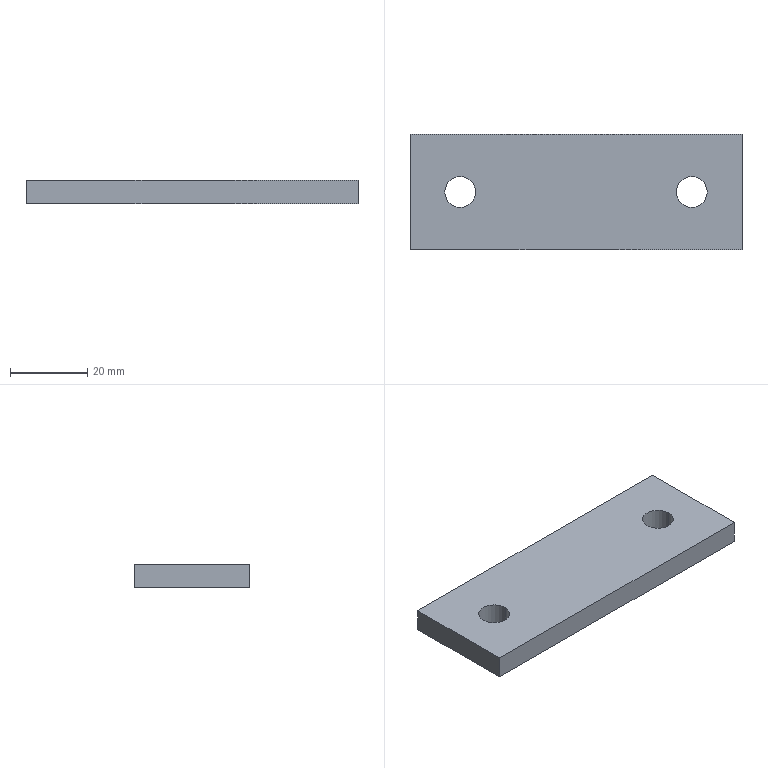Part | SolidWorks | features Extrusion 1, ICE 1 | 1 solid | 10 faces | box 86 x 30 x 6 mm | volume 14877 mm3 | plane 6 | cylinder 4 | commonest cylinder face diameters 8 x4
STEP:
#1=CARTESIAN_POINT('',(-26.,0.,0.));
#2=VERTEX_POINT('',#1);
#3=CARTESIAN_POINT('',(-34.,0.,0.));
#4=VERTEX_POINT('',#3);
#5=CARTESIAN_POINT('',(-30.,0.,0.));
#6=DIRECTION('',(0.,0.,-1.));
#7=DIRECTION('',(-1.,0.,0.));
#8=AXIS2_PLACEMENT_3D('',#5,#6,#7);
#9=CIRCLE('',#8,4.);
#10=EDGE_CURVE('',#2,#4,#9,.T.);
#11=ORIENTED_EDGE('',*,*,#10,.T.);
#12=CARTESIAN_POINT('',(-34.,0.,6.));
#13=VERTEX_POINT('',#12);
#14=CARTESIAN_POINT('',(-34.,0.,-4.));
#15=DIRECTION('',(0.,0.,1.));
#16=VECTOR('',#15,1000.);
#17=LINE('',#14,#16);
#18=EDGE_CURVE('',#4,#13,#17,.T.);
#19=ORIENTED_EDGE('',*,*,#18,.T.);
#20=CARTESIAN_POINT('',(-26.,0.,6.));
#21=VERTEX_POINT('',#20);
#22=CARTESIAN_POINT('',(-30.,0.,6.));
#23=DIRECTION('',(0.,0.,1.));
#24=DIRECTION('',(1.,0.,0.));
#25=AXIS2_PLACEMENT_3D('',#22,#23,#24);
#26=CIRCLE('',#25,4.);
#27=EDGE_CURVE('',#13,#21,#26,.T.);
#28=ORIENTED_EDGE('',*,*,#27,.T.);
#29=CARTESIAN_POINT('',(-26.,0.,-4.));
#30=DIRECTION('',(0.,0.,1.));
#31=VECTOR('',#30,1000.);
#32=LINE('',#29,#31);
#33=EDGE_CURVE('',#2,#21,#32,.T.);
#34=ORIENTED_EDGE('',*,*,#33,.F.);
#35=EDGE_LOOP('',(#11,#19,#28,#34));
#36=FACE_OUTER_BOUND('',#35,.T.);
#37=CARTESIAN_POINT('',(-30.,0.,-4.));
#38=DIRECTION('',(0.,0.,1.));
#39=DIRECTION('',(1.,0.,0.));
#40=AXIS2_PLACEMENT_3D('',#37,#38,#39);
#41=CYLINDRICAL_SURFACE('',#40,4.);
#42=ADVANCED_FACE('',(#36),#41,.F.);
#43=CARTESIAN_POINT('',(34.,0.,0.));
#44=VERTEX_POINT('',#43);
#45=CARTESIAN_POINT('',(26.,0.,0.));
#46=VERTEX_POINT('',#45);
#47=CARTESIAN_POINT('',(30.,0.,0.));
#48=DIRECTION('',(0.,0.,-1.));
#49=DIRECTION('',(-1.,0.,0.));
#50=AXIS2_PLACEMENT_3D('',#47,#48,#49);
#51=CIRCLE('',#50,4.);
#52=EDGE_CURVE('',#44,#46,#51,.T.);
#53=ORIENTED_EDGE('',*,*,#52,.T.);
#54=CARTESIAN_POINT('',(26.,0.,6.));
#55=VERTEX_POINT('',#54);
#56=CARTESIAN_POINT('',(26.,0.,-4.));
#57=DIRECTION('',(0.,0.,1.));
#58=VECTOR('',#57,1000.);
#59=LINE('',#56,#58);
#60=EDGE_CURVE('',#46,#55,#59,.T.);
#61=ORIENTED_EDGE('',*,*,#60,.T.);
#62=CARTESIAN_POINT('',(34.,0.,6.));
#63=VERTEX_POINT('',#62);
#64=CARTESIAN_POINT('',(30.,0.,6.));
#65=DIRECTION('',(0.,0.,1.));
#66=DIRECTION('',(1.,0.,0.));
#67=AXIS2_PLACEMENT_3D('',#64,#65,#66);
#68=CIRCLE('',#67,4.);
#69=EDGE_CURVE('',#55,#63,#68,.T.);
#70=ORIENTED_EDGE('',*,*,#69,.T.);
#71=CARTESIAN_POINT('',(34.,0.,-4.));
#72=DIRECTION('',(0.,0.,1.));
#73=VECTOR('',#72,1000.);
#74=LINE('',#71,#73);
#75=EDGE_CURVE('',#44,#63,#74,.T.);
#76=ORIENTED_EDGE('',*,*,#75,.F.);
#77=EDGE_LOOP('',(#53,#61,#70,#76));
#78=FACE_OUTER_BOUND('',#77,.T.);
#79=CARTESIAN_POINT('',(30.,0.,-4.));
#80=DIRECTION('',(0.,0.,1.));
#81=DIRECTION('',(1.,0.,0.));
#82=AXIS2_PLACEMENT_3D('',#79,#80,#81);
#83=CYLINDRICAL_SURFACE('',#82,4.);
#84=ADVANCED_FACE('',(#78),#83,.F.);
#85=CARTESIAN_POINT('',(-43.,15.,0.));
#86=VERTEX_POINT('',#85);
#87=CARTESIAN_POINT('',(-43.,-15.,0.));
#88=VERTEX_POINT('',#87);
#89=CARTESIAN_POINT('',(-43.,15.,0.));
#90=DIRECTION('',(0.,-1.,0.));
#91=VECTOR('',#90,1000.);
#92=LINE('',#89,#91);
#93=EDGE_CURVE('',#86,#88,#92,.T.);
#94=ORIENTED_EDGE('',*,*,#93,.T.);
#95=CARTESIAN_POINT('',(-43.,-15.,6.));
#96=VERTEX_POINT('',#95);
#97=CARTESIAN_POINT('',(-43.,-15.,6.));
#98=DIRECTION('',(0.,0.,-1.));
#99=VECTOR('',#98,1000.);
#100=LINE('',#97,#99);
#101=EDGE_CURVE('',#96,#88,#100,.T.);
#102=ORIENTED_EDGE('',*,*,#101,.F.);
#103=CARTESIAN_POINT('',(-43.,15.,6.));
#104=VERTEX_POINT('',#103);
#105=CARTESIAN_POINT('',(-43.,15.,6.));
#106=DIRECTION('',(0.,-1.,0.));
#107=VECTOR('',#106,1000.);
#108=LINE('',#105,#107);
#109=EDGE_CURVE('',#104,#96,#108,.T.);
#110=ORIENTED_EDGE('',*,*,#109,.F.);
#111=CARTESIAN_POINT('',(-43.,15.,6.));
#112=DIRECTION('',(0.,0.,-1.));
#113=VECTOR('',#112,1000.);
#114=LINE('',#111,#113);
#115=EDGE_CURVE('',#104,#86,#114,.T.);
#116=ORIENTED_EDGE('',*,*,#115,.T.);
#117=EDGE_LOOP('',(#94,#102,#110,#116));
#118=FACE_OUTER_BOUND('',#117,.T.);
#119=CARTESIAN_POINT('',(-43.,15.,6.));
#120=DIRECTION('',(1.,0.,0.));
#121=DIRECTION('',(0.,1.,0.));
#122=AXIS2_PLACEMENT_3D('',#119,#120,#121);
#123=PLANE('',#122);
#124=ADVANCED_FACE('',(#118),#123,.F.);
#125=CARTESIAN_POINT('',(43.,-15.,0.));
#126=VERTEX_POINT('',#125);
#127=CARTESIAN_POINT('',(43.,-15.,0.));
#128=DIRECTION('',(1.,0.,0.));
#129=VECTOR('',#128,1000.);
#130=LINE('',#127,#129);
#131=EDGE_CURVE('',#88,#126,#130,.T.);
#132=ORIENTED_EDGE('',*,*,#131,.T.);
#133=CARTESIAN_POINT('',(43.,-15.,6.));
#134=VERTEX_POINT('',#133);
#135=CARTESIAN_POINT('',(43.,-15.,6.));
#136=DIRECTION('',(0.,0.,-1.));
#137=VECTOR('',#136,1000.);
#138=LINE('',#135,#137);
#139=EDGE_CURVE('',#134,#126,#138,.T.);
#140=ORIENTED_EDGE('',*,*,#139,.F.);
#141=CARTESIAN_POINT('',(43.,-15.,6.));
#142=DIRECTION('',(1.,0.,0.));
#143=VECTOR('',#142,1000.);
#144=LINE('',#141,#143);
#145=EDGE_CURVE('',#96,#134,#144,.T.);
#146=ORIENTED_EDGE('',*,*,#145,.F.);
#147=ORIENTED_EDGE('',*,*,#101,.T.);
#148=EDGE_LOOP('',(#132,#140,#146,#147));
#149=FACE_OUTER_BOUND('',#148,.T.);
#150=CARTESIAN_POINT('',(43.,-15.,6.));
#151=DIRECTION('',(0.,1.,0.));
#152=DIRECTION('',(-1.,0.,0.));
#153=AXIS2_PLACEMENT_3D('',#150,#151,#152);
#154=PLANE('',#153);
#155=ADVANCED_FACE('',(#149),#154,.F.);
#156=CARTESIAN_POINT('',(43.,15.,0.));
#157=VERTEX_POINT('',#156);
#158=CARTESIAN_POINT('',(43.,15.,0.));
#159=DIRECTION('',(0.,1.,0.));
#160=VECTOR('',#159,1000.);
#161=LINE('',#158,#160);
#162=EDGE_CURVE('',#126,#157,#161,.T.);
#163=ORIENTED_EDGE('',*,*,#162,.T.);
#164=CARTESIAN_POINT('',(43.,15.,6.));
#165=VERTEX_POINT('',#164);
#166=CARTESIAN_POINT('',(43.,15.,6.));
#167=DIRECTION('',(0.,0.,-1.));
#168=VECTOR('',#167,1000.);
#169=LINE('',#166,#168);
#170=EDGE_CURVE('',#165,#157,#169,.T.);
#171=ORIENTED_EDGE('',*,*,#170,.F.);
#172=CARTESIAN_POINT('',(43.,15.,6.));
#173=DIRECTION('',(0.,1.,0.));
#174=VECTOR('',#173,1000.);
#175=LINE('',#172,#174);
#176=EDGE_CURVE('',#134,#165,#175,.T.);
#177=ORIENTED_EDGE('',*,*,#176,.F.);
#178=ORIENTED_EDGE('',*,*,#139,.T.);
#179=EDGE_LOOP('',(#163,#171,#177,#178));
#180=FACE_OUTER_BOUND('',#179,.T.);
#181=CARTESIAN_POINT('',(43.,15.,6.));
#182=DIRECTION('',(-1.,0.,0.));
#183=DIRECTION('',(0.,-1.,0.));
#184=AXIS2_PLACEMENT_3D('',#181,#182,#183);
#185=PLANE('',#184);
#186=ADVANCED_FACE('',(#180),#185,.F.);
#187=CARTESIAN_POINT('',(43.,15.,0.));
#188=DIRECTION('',(-1.,0.,0.));
#189=VECTOR('',#188,1000.);
#190=LINE('',#187,#189);
#191=EDGE_CURVE('',#157,#86,#190,.T.);
#192=ORIENTED_EDGE('',*,*,#191,.T.);
#193=ORIENTED_EDGE('',*,*,#115,.F.);
#194=CARTESIAN_POINT('',(43.,15.,6.));
#195=DIRECTION('',(-1.,0.,0.));
#196=VECTOR('',#195,1000.);
#197=LINE('',#194,#196);
#198=EDGE_CURVE('',#165,#104,#197,.T.);
#199=ORIENTED_EDGE('',*,*,#198,.F.);
#200=ORIENTED_EDGE('',*,*,#170,.T.);
#201=EDGE_LOOP('',(#192,#193,#199,#200));
#202=FACE_OUTER_BOUND('',#201,.T.);
#203=CARTESIAN_POINT('',(43.,15.,6.));
#204=DIRECTION('',(0.,-1.,0.));
#205=DIRECTION('',(1.,0.,0.));
#206=AXIS2_PLACEMENT_3D('',#203,#204,#205);
#207=PLANE('',#206);
#208=ADVANCED_FACE('',(#202),#207,.F.);
#209=CARTESIAN_POINT('',(-30.,0.,6.));
#210=DIRECTION('',(0.,0.,1.));
#211=DIRECTION('',(1.,0.,0.));
#212=AXIS2_PLACEMENT_3D('',#209,#210,#211);
#213=CIRCLE('',#212,4.);
#214=EDGE_CURVE('',#21,#13,#213,.T.);
#215=ORIENTED_EDGE('',*,*,#214,.F.);
#216=ORIENTED_EDGE('',*,*,#27,.F.);
#217=EDGE_LOOP('',(#215,#216));
#218=FACE_BOUND('',#217,.T.);
#219=CARTESIAN_POINT('',(30.,0.,6.));
#220=DIRECTION('',(0.,0.,1.));
#221=DIRECTION('',(1.,0.,0.));
#222=AXIS2_PLACEMENT_3D('',#219,#220,#221);
#223=CIRCLE('',#222,4.);
#224=EDGE_CURVE('',#63,#55,#223,.T.);
#225=ORIENTED_EDGE('',*,*,#224,.F.);
#226=ORIENTED_EDGE('',*,*,#69,.F.);
#227=EDGE_LOOP('',(#225,#226));
#228=FACE_BOUND('',#227,.T.);
#229=ORIENTED_EDGE('',*,*,#109,.T.);
#230=ORIENTED_EDGE('',*,*,#145,.T.);
#231=ORIENTED_EDGE('',*,*,#176,.T.);
#232=ORIENTED_EDGE('',*,*,#198,.T.);
#233=EDGE_LOOP('',(#229,#230,#231,#232));
#234=FACE_OUTER_BOUND('',#233,.T.);
#235=CARTESIAN_POINT('',(0.,0.,6.));
#236=DIRECTION('',(0.,0.,-1.));
#237=DIRECTION('',(-1.,0.,0.));
#238=AXIS2_PLACEMENT_3D('',#235,#236,#237);
#239=PLANE('',#238);
#240=ADVANCED_FACE('',(#218,#228,#234),#239,.F.);
#241=ORIENTED_EDGE('',*,*,#10,.F.);
#242=CARTESIAN_POINT('',(-30.,0.,0.));
#243=DIRECTION('',(0.,0.,-1.));
#244=DIRECTION('',(-1.,0.,0.));
#245=AXIS2_PLACEMENT_3D('',#242,#243,#244);
#246=CIRCLE('',#245,4.);
#247=EDGE_CURVE('',#4,#2,#246,.T.);
#248=ORIENTED_EDGE('',*,*,#247,.F.);
#249=EDGE_LOOP('',(#241,#248));
#250=FACE_BOUND('',#249,.T.);
#251=ORIENTED_EDGE('',*,*,#52,.F.);
#252=CARTESIAN_POINT('',(30.,0.,0.));
#253=DIRECTION('',(0.,0.,-1.));
#254=DIRECTION('',(-1.,0.,0.));
#255=AXIS2_PLACEMENT_3D('',#252,#253,#254);
#256=CIRCLE('',#255,4.);
#257=EDGE_CURVE('',#46,#44,#256,.T.);
#258=ORIENTED_EDGE('',*,*,#257,.F.);
#259=EDGE_LOOP('',(#251,#258));
#260=FACE_BOUND('',#259,.T.);
#261=ORIENTED_EDGE('',*,*,#93,.F.);
#262=ORIENTED_EDGE('',*,*,#191,.F.);
#263=ORIENTED_EDGE('',*,*,#162,.F.);
#264=ORIENTED_EDGE('',*,*,#131,.F.);
#265=EDGE_LOOP('',(#261,#262,#263,#264));
#266=FACE_OUTER_BOUND('',#265,.T.);
#267=CARTESIAN_POINT('',(0.,0.,0.));
#268=DIRECTION('',(0.,0.,-1.));
#269=DIRECTION('',(-1.,0.,0.));
#270=AXIS2_PLACEMENT_3D('',#267,#268,#269);
#271=PLANE('',#270);
#272=ADVANCED_FACE('',(#250,#260,#266),#271,.T.);
#273=ORIENTED_EDGE('',*,*,#60,.F.);
#274=ORIENTED_EDGE('',*,*,#257,.T.);
#275=ORIENTED_EDGE('',*,*,#75,.T.);
#276=ORIENTED_EDGE('',*,*,#224,.T.);
#277=EDGE_LOOP('',(#273,#274,#275,#276));
#278=FACE_OUTER_BOUND('',#277,.T.);
#279=CARTESIAN_POINT('',(30.,0.,-4.));
#280=DIRECTION('',(0.,0.,1.));
#281=DIRECTION('',(1.,0.,0.));
#282=AXIS2_PLACEMENT_3D('',#279,#280,#281);
#283=CYLINDRICAL_SURFACE('',#282,4.);
#284=ADVANCED_FACE('',(#278),#283,.F.);
#285=ORIENTED_EDGE('',*,*,#18,.F.);
#286=ORIENTED_EDGE('',*,*,#247,.T.);
#287=ORIENTED_EDGE('',*,*,#33,.T.);
#288=ORIENTED_EDGE('',*,*,#214,.T.);
#289=EDGE_LOOP('',(#285,#286,#287,#288));
#290=FACE_OUTER_BOUND('',#289,.T.);
#291=CARTESIAN_POINT('',(-30.,0.,-4.));
#292=DIRECTION('',(0.,0.,1.));
#293=DIRECTION('',(1.,0.,0.));
#294=AXIS2_PLACEMENT_3D('',#291,#292,#293);
#295=CYLINDRICAL_SURFACE('',#294,4.);
#296=ADVANCED_FACE('',(#290),#295,.F.);
#297=CLOSED_SHELL('',(#42,#84,#124,#155,#186,#208,#240,#272,#284,#296));
#298=MANIFOLD_SOLID_BREP('',#297);
#299=CARTESIAN_POINT('',(0.,0.,0.));
#300=DIRECTION('',(0.,0.,1.));
#301=DIRECTION('',(1.,0.,0.));
#302=AXIS2_PLACEMENT_3D('',#299,#300,#301);
#303=(LENGTH_UNIT()NAMED_UNIT(*)SI_UNIT(.MILLI.,.METRE.));
#304=UNCERTAINTY_MEASURE_WITH_UNIT(LENGTH_MEASURE(0.00001),#303,'','');
#305=(NAMED_UNIT(*)PLANE_ANGLE_UNIT()SI_UNIT($,.RADIAN.));
#306=(NAMED_UNIT(*)SI_UNIT($,.STERADIAN.)SOLID_ANGLE_UNIT());
#307=(GEOMETRIC_REPRESENTATION_CONTEXT(3)GLOBAL_UNCERTAINTY_ASSIGNED_CONTEXT((#304))GLOBAL_UNIT_ASSIGNED_CONTEXT((#303,#305,#306))REPRESENTATION_CONTEXT('',''));
#308=ADVANCED_BREP_SHAPE_REPRESENTATION('',(#298,#302),#307);